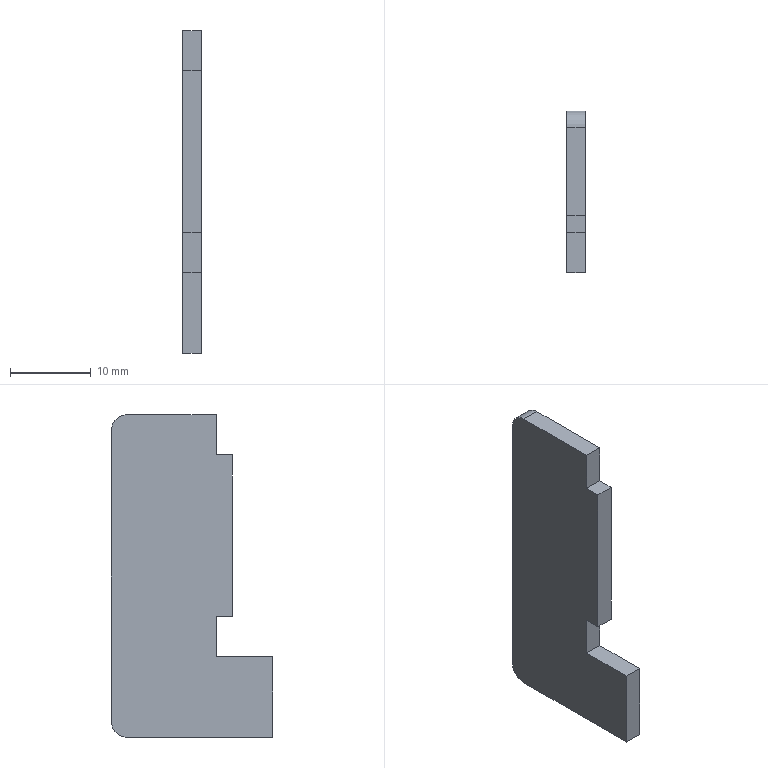Part | SolidWorks | features FlatPattern 1, SMBaseFlange 1, SheetMetal 1 | 1 solid | 14 faces | box 2.3 x 20 x 40 mm | volume 1445 mm3 | plane 12 | cylinder 2 | commonest cylinder face diameters 4 x2
STEP:
#1=CARTESIAN_POINT('',(0.,0.,10.));
#2=VERTEX_POINT('',#1);
#3=CARTESIAN_POINT('',(0.,0.,0.));
#4=VERTEX_POINT('',#3);
#5=CARTESIAN_POINT('',(0.,0.,10.));
#6=DIRECTION('',(0.,0.,-1.));
#7=VECTOR('',#6,1000.);
#8=LINE('',#5,#7);
#9=EDGE_CURVE('',#2,#4,#8,.T.);
#10=ORIENTED_EDGE('',*,*,#9,.F.);
#11=CARTESIAN_POINT('',(-2.3,0.,10.));
#12=VERTEX_POINT('',#11);
#13=CARTESIAN_POINT('',(-2.3,0.,10.));
#14=DIRECTION('',(1.,0.,0.));
#15=VECTOR('',#14,1000.);
#16=LINE('',#13,#15);
#17=EDGE_CURVE('',#12,#2,#16,.T.);
#18=ORIENTED_EDGE('',*,*,#17,.F.);
#19=CARTESIAN_POINT('',(-2.3,0.,0.));
#20=VERTEX_POINT('',#19);
#21=CARTESIAN_POINT('',(-2.3,0.,10.));
#22=DIRECTION('',(0.,0.,-1.));
#23=VECTOR('',#22,1000.);
#24=LINE('',#21,#23);
#25=EDGE_CURVE('',#12,#20,#24,.T.);
#26=ORIENTED_EDGE('',*,*,#25,.T.);
#27=CARTESIAN_POINT('',(-2.3,0.,0.));
#28=DIRECTION('',(1.,0.,0.));
#29=VECTOR('',#28,1000.);
#30=LINE('',#27,#29);
#31=EDGE_CURVE('',#20,#4,#30,.T.);
#32=ORIENTED_EDGE('',*,*,#31,.T.);
#33=EDGE_LOOP('',(#10,#18,#26,#32));
#34=FACE_OUTER_BOUND('',#33,.T.);
#35=CARTESIAN_POINT('',(-2.3,0.,10.));
#36=DIRECTION('',(0.,-1.,0.));
#37=DIRECTION('',(0.,0.,-1.));
#38=AXIS2_PLACEMENT_3D('',#35,#36,#37);
#39=PLANE('',#38);
#40=ADVANCED_FACE('',(#34),#39,.T.);
#41=CARTESIAN_POINT('',(0.,7.,10.));
#42=VERTEX_POINT('',#41);
#43=CARTESIAN_POINT('',(0.,7.,10.));
#44=DIRECTION('',(0.,-1.,0.));
#45=VECTOR('',#44,1000.);
#46=LINE('',#43,#45);
#47=EDGE_CURVE('',#42,#2,#46,.T.);
#48=ORIENTED_EDGE('',*,*,#47,.F.);
#49=CARTESIAN_POINT('',(-2.3,7.,10.));
#50=VERTEX_POINT('',#49);
#51=CARTESIAN_POINT('',(-2.3,7.,10.));
#52=DIRECTION('',(1.,0.,0.));
#53=VECTOR('',#52,1000.);
#54=LINE('',#51,#53);
#55=EDGE_CURVE('',#50,#42,#54,.T.);
#56=ORIENTED_EDGE('',*,*,#55,.F.);
#57=CARTESIAN_POINT('',(-2.3,7.,10.));
#58=DIRECTION('',(0.,-1.,0.));
#59=VECTOR('',#58,1000.);
#60=LINE('',#57,#59);
#61=EDGE_CURVE('',#50,#12,#60,.T.);
#62=ORIENTED_EDGE('',*,*,#61,.T.);
#63=ORIENTED_EDGE('',*,*,#17,.T.);
#64=EDGE_LOOP('',(#48,#56,#62,#63));
#65=FACE_OUTER_BOUND('',#64,.T.);
#66=CARTESIAN_POINT('',(-2.3,7.,10.));
#67=DIRECTION('',(0.,0.,1.));
#68=DIRECTION('',(0.,-1.,0.));
#69=AXIS2_PLACEMENT_3D('',#66,#67,#68);
#70=PLANE('',#69);
#71=ADVANCED_FACE('',(#65),#70,.T.);
#72=CARTESIAN_POINT('',(0.,7.,15.));
#73=VERTEX_POINT('',#72);
#74=CARTESIAN_POINT('',(0.,7.,15.));
#75=DIRECTION('',(0.,0.,-1.));
#76=VECTOR('',#75,1000.);
#77=LINE('',#74,#76);
#78=EDGE_CURVE('',#73,#42,#77,.T.);
#79=ORIENTED_EDGE('',*,*,#78,.F.);
#80=CARTESIAN_POINT('',(-2.3,7.,15.));
#81=VERTEX_POINT('',#80);
#82=CARTESIAN_POINT('',(-2.3,7.,15.));
#83=DIRECTION('',(1.,0.,0.));
#84=VECTOR('',#83,1000.);
#85=LINE('',#82,#84);
#86=EDGE_CURVE('',#81,#73,#85,.T.);
#87=ORIENTED_EDGE('',*,*,#86,.F.);
#88=CARTESIAN_POINT('',(-2.3,7.,15.));
#89=DIRECTION('',(0.,0.,-1.));
#90=VECTOR('',#89,1000.);
#91=LINE('',#88,#90);
#92=EDGE_CURVE('',#81,#50,#91,.T.);
#93=ORIENTED_EDGE('',*,*,#92,.T.);
#94=ORIENTED_EDGE('',*,*,#55,.T.);
#95=EDGE_LOOP('',(#79,#87,#93,#94));
#96=FACE_OUTER_BOUND('',#95,.T.);
#97=CARTESIAN_POINT('',(-2.3,7.,15.));
#98=DIRECTION('',(0.,-1.,0.));
#99=DIRECTION('',(0.,0.,-1.));
#100=AXIS2_PLACEMENT_3D('',#97,#98,#99);
#101=PLANE('',#100);
#102=ADVANCED_FACE('',(#96),#101,.T.);
#103=CARTESIAN_POINT('',(0.,5.,15.));
#104=VERTEX_POINT('',#103);
#105=CARTESIAN_POINT('',(0.,5.,15.));
#106=DIRECTION('',(0.,1.,0.));
#107=VECTOR('',#106,1000.);
#108=LINE('',#105,#107);
#109=EDGE_CURVE('',#104,#73,#108,.T.);
#110=ORIENTED_EDGE('',*,*,#109,.F.);
#111=CARTESIAN_POINT('',(-2.3,5.,15.));
#112=VERTEX_POINT('',#111);
#113=CARTESIAN_POINT('',(-2.3,5.,15.));
#114=DIRECTION('',(1.,0.,0.));
#115=VECTOR('',#114,1000.);
#116=LINE('',#113,#115);
#117=EDGE_CURVE('',#112,#104,#116,.T.);
#118=ORIENTED_EDGE('',*,*,#117,.F.);
#119=CARTESIAN_POINT('',(-2.3,5.,15.));
#120=DIRECTION('',(0.,1.,0.));
#121=VECTOR('',#120,1000.);
#122=LINE('',#119,#121);
#123=EDGE_CURVE('',#112,#81,#122,.T.);
#124=ORIENTED_EDGE('',*,*,#123,.T.);
#125=ORIENTED_EDGE('',*,*,#86,.T.);
#126=EDGE_LOOP('',(#110,#118,#124,#125));
#127=FACE_OUTER_BOUND('',#126,.T.);
#128=CARTESIAN_POINT('',(-2.3,5.,15.));
#129=DIRECTION('',(0.,0.,-1.));
#130=DIRECTION('',(-1.,0.,0.));
#131=AXIS2_PLACEMENT_3D('',#128,#129,#130);
#132=PLANE('',#131);
#133=ADVANCED_FACE('',(#127),#132,.T.);
#134=CARTESIAN_POINT('',(0.,5.,35.));
#135=VERTEX_POINT('',#134);
#136=CARTESIAN_POINT('',(0.,5.,35.));
#137=DIRECTION('',(0.,0.,-1.));
#138=VECTOR('',#137,1000.);
#139=LINE('',#136,#138);
#140=EDGE_CURVE('',#135,#104,#139,.T.);
#141=ORIENTED_EDGE('',*,*,#140,.F.);
#142=CARTESIAN_POINT('',(-2.3,5.,35.));
#143=VERTEX_POINT('',#142);
#144=CARTESIAN_POINT('',(-2.3,5.,35.));
#145=DIRECTION('',(1.,0.,0.));
#146=VECTOR('',#145,1000.);
#147=LINE('',#144,#146);
#148=EDGE_CURVE('',#143,#135,#147,.T.);
#149=ORIENTED_EDGE('',*,*,#148,.F.);
#150=CARTESIAN_POINT('',(-2.3,5.,35.));
#151=DIRECTION('',(0.,0.,-1.));
#152=VECTOR('',#151,1000.);
#153=LINE('',#150,#152);
#154=EDGE_CURVE('',#143,#112,#153,.T.);
#155=ORIENTED_EDGE('',*,*,#154,.T.);
#156=ORIENTED_EDGE('',*,*,#117,.T.);
#157=EDGE_LOOP('',(#141,#149,#155,#156));
#158=FACE_OUTER_BOUND('',#157,.T.);
#159=CARTESIAN_POINT('',(-2.3,5.,35.));
#160=DIRECTION('',(0.,-1.,0.));
#161=DIRECTION('',(0.,0.,-1.));
#162=AXIS2_PLACEMENT_3D('',#159,#160,#161);
#163=PLANE('',#162);
#164=ADVANCED_FACE('',(#158),#163,.T.);
#165=CARTESIAN_POINT('',(0.,7.,35.));
#166=VERTEX_POINT('',#165);
#167=CARTESIAN_POINT('',(0.,7.,35.));
#168=DIRECTION('',(0.,-1.,0.));
#169=VECTOR('',#168,1000.);
#170=LINE('',#167,#169);
#171=EDGE_CURVE('',#166,#135,#170,.T.);
#172=ORIENTED_EDGE('',*,*,#171,.F.);
#173=CARTESIAN_POINT('',(-2.3,7.,35.));
#174=VERTEX_POINT('',#173);
#175=CARTESIAN_POINT('',(-2.3,7.,35.));
#176=DIRECTION('',(1.,0.,0.));
#177=VECTOR('',#176,1000.);
#178=LINE('',#175,#177);
#179=EDGE_CURVE('',#174,#166,#178,.T.);
#180=ORIENTED_EDGE('',*,*,#179,.F.);
#181=CARTESIAN_POINT('',(-2.3,7.,35.));
#182=DIRECTION('',(0.,-1.,0.));
#183=VECTOR('',#182,1000.);
#184=LINE('',#181,#183);
#185=EDGE_CURVE('',#174,#143,#184,.T.);
#186=ORIENTED_EDGE('',*,*,#185,.T.);
#187=ORIENTED_EDGE('',*,*,#148,.T.);
#188=EDGE_LOOP('',(#172,#180,#186,#187));
#189=FACE_OUTER_BOUND('',#188,.T.);
#190=CARTESIAN_POINT('',(-2.3,7.,35.));
#191=DIRECTION('',(0.,0.,1.));
#192=DIRECTION('',(1.,0.,0.));
#193=AXIS2_PLACEMENT_3D('',#190,#191,#192);
#194=PLANE('',#193);
#195=ADVANCED_FACE('',(#189),#194,.T.);
#196=CARTESIAN_POINT('',(0.,7.,40.));
#197=VERTEX_POINT('',#196);
#198=CARTESIAN_POINT('',(0.,7.,40.));
#199=DIRECTION('',(0.,0.,-1.));
#200=VECTOR('',#199,1000.);
#201=LINE('',#198,#200);
#202=EDGE_CURVE('',#197,#166,#201,.T.);
#203=ORIENTED_EDGE('',*,*,#202,.F.);
#204=CARTESIAN_POINT('',(-2.3,7.,40.));
#205=VERTEX_POINT('',#204);
#206=CARTESIAN_POINT('',(-2.3,7.,40.));
#207=DIRECTION('',(1.,0.,0.));
#208=VECTOR('',#207,1000.);
#209=LINE('',#206,#208);
#210=EDGE_CURVE('',#205,#197,#209,.T.);
#211=ORIENTED_EDGE('',*,*,#210,.F.);
#212=CARTESIAN_POINT('',(-2.3,7.,40.));
#213=DIRECTION('',(0.,0.,-1.));
#214=VECTOR('',#213,1000.);
#215=LINE('',#212,#214);
#216=EDGE_CURVE('',#205,#174,#215,.T.);
#217=ORIENTED_EDGE('',*,*,#216,.T.);
#218=ORIENTED_EDGE('',*,*,#179,.T.);
#219=EDGE_LOOP('',(#203,#211,#217,#218));
#220=FACE_OUTER_BOUND('',#219,.T.);
#221=CARTESIAN_POINT('',(-2.3,7.,40.));
#222=DIRECTION('',(0.,-1.,0.));
#223=DIRECTION('',(0.,0.,-1.));
#224=AXIS2_PLACEMENT_3D('',#221,#222,#223);
#225=PLANE('',#224);
#226=ADVANCED_FACE('',(#220),#225,.T.);
#227=CARTESIAN_POINT('',(0.,18.,40.));
#228=VERTEX_POINT('',#227);
#229=CARTESIAN_POINT('',(0.,18.,40.));
#230=DIRECTION('',(0.,-1.,0.));
#231=VECTOR('',#230,1000.);
#232=LINE('',#229,#231);
#233=EDGE_CURVE('',#228,#197,#232,.T.);
#234=ORIENTED_EDGE('',*,*,#233,.F.);
#235=CARTESIAN_POINT('',(-2.3,18.,40.));
#236=VERTEX_POINT('',#235);
#237=CARTESIAN_POINT('',(-2.3,18.,40.));
#238=DIRECTION('',(1.,0.,0.));
#239=VECTOR('',#238,1000.);
#240=LINE('',#237,#239);
#241=EDGE_CURVE('',#236,#228,#240,.T.);
#242=ORIENTED_EDGE('',*,*,#241,.F.);
#243=CARTESIAN_POINT('',(-2.3,18.,40.));
#244=DIRECTION('',(0.,-1.,0.));
#245=VECTOR('',#244,1000.);
#246=LINE('',#243,#245);
#247=EDGE_CURVE('',#236,#205,#246,.T.);
#248=ORIENTED_EDGE('',*,*,#247,.T.);
#249=ORIENTED_EDGE('',*,*,#210,.T.);
#250=EDGE_LOOP('',(#234,#242,#248,#249));
#251=FACE_OUTER_BOUND('',#250,.T.);
#252=CARTESIAN_POINT('',(-2.3,18.,40.));
#253=DIRECTION('',(0.,0.,1.));
#254=DIRECTION('',(1.,0.,0.));
#255=AXIS2_PLACEMENT_3D('',#252,#253,#254);
#256=PLANE('',#255);
#257=ADVANCED_FACE('',(#251),#256,.T.);
#258=CARTESIAN_POINT('',(0.,20.,38.));
#259=VERTEX_POINT('',#258);
#260=CARTESIAN_POINT('',(0.,18.,38.));
#261=DIRECTION('',(1.,0.,0.));
#262=DIRECTION('',(0.,0.,-1.));
#263=AXIS2_PLACEMENT_3D('',#260,#261,#262);
#264=CIRCLE('',#263,2.);
#265=EDGE_CURVE('',#259,#228,#264,.T.);
#266=ORIENTED_EDGE('',*,*,#265,.F.);
#267=CARTESIAN_POINT('',(-2.3,20.,38.));
#268=VERTEX_POINT('',#267);
#269=CARTESIAN_POINT('',(-2.3,20.,38.));
#270=DIRECTION('',(1.,0.,0.));
#271=VECTOR('',#270,1000.);
#272=LINE('',#269,#271);
#273=EDGE_CURVE('',#268,#259,#272,.T.);
#274=ORIENTED_EDGE('',*,*,#273,.F.);
#275=CARTESIAN_POINT('',(-2.3,18.,38.));
#276=DIRECTION('',(1.,0.,0.));
#277=DIRECTION('',(0.,0.,-1.));
#278=AXIS2_PLACEMENT_3D('',#275,#276,#277);
#279=CIRCLE('',#278,2.);
#280=EDGE_CURVE('',#268,#236,#279,.T.);
#281=ORIENTED_EDGE('',*,*,#280,.T.);
#282=ORIENTED_EDGE('',*,*,#241,.T.);
#283=EDGE_LOOP('',(#266,#274,#281,#282));
#284=FACE_OUTER_BOUND('',#283,.T.);
#285=CARTESIAN_POINT('',(-2.3,18.,38.));
#286=DIRECTION('',(1.,0.,0.));
#287=DIRECTION('',(0.,0.,-1.));
#288=AXIS2_PLACEMENT_3D('',#285,#286,#287);
#289=CYLINDRICAL_SURFACE('',#288,2.);
#290=ADVANCED_FACE('',(#284),#289,.T.);
#291=CARTESIAN_POINT('',(0.,20.,2.));
#292=VERTEX_POINT('',#291);
#293=CARTESIAN_POINT('',(0.,20.,2.));
#294=DIRECTION('',(0.,0.,1.));
#295=VECTOR('',#294,1000.);
#296=LINE('',#293,#295);
#297=EDGE_CURVE('',#292,#259,#296,.T.);
#298=ORIENTED_EDGE('',*,*,#297,.F.);
#299=CARTESIAN_POINT('',(-2.3,20.,2.));
#300=VERTEX_POINT('',#299);
#301=CARTESIAN_POINT('',(-2.3,20.,2.));
#302=DIRECTION('',(1.,0.,0.));
#303=VECTOR('',#302,1000.);
#304=LINE('',#301,#303);
#305=EDGE_CURVE('',#300,#292,#304,.T.);
#306=ORIENTED_EDGE('',*,*,#305,.F.);
#307=CARTESIAN_POINT('',(-2.3,20.,2.));
#308=DIRECTION('',(0.,0.,1.));
#309=VECTOR('',#308,1000.);
#310=LINE('',#307,#309);
#311=EDGE_CURVE('',#300,#268,#310,.T.);
#312=ORIENTED_EDGE('',*,*,#311,.T.);
#313=ORIENTED_EDGE('',*,*,#273,.T.);
#314=EDGE_LOOP('',(#298,#306,#312,#313));
#315=FACE_OUTER_BOUND('',#314,.T.);
#316=CARTESIAN_POINT('',(-2.3,20.,2.));
#317=DIRECTION('',(0.,1.,0.));
#318=DIRECTION('',(0.,0.,1.));
#319=AXIS2_PLACEMENT_3D('',#316,#317,#318);
#320=PLANE('',#319);
#321=ADVANCED_FACE('',(#315),#320,.T.);
#322=CARTESIAN_POINT('',(0.,18.,0.));
#323=VERTEX_POINT('',#322);
#324=CARTESIAN_POINT('',(0.,18.,2.));
#325=DIRECTION('',(1.,0.,0.));
#326=DIRECTION('',(0.,0.,-1.));
#327=AXIS2_PLACEMENT_3D('',#324,#325,#326);
#328=CIRCLE('',#327,2.);
#329=EDGE_CURVE('',#323,#292,#328,.T.);
#330=ORIENTED_EDGE('',*,*,#329,.F.);
#331=CARTESIAN_POINT('',(-2.3,18.,0.));
#332=VERTEX_POINT('',#331);
#333=CARTESIAN_POINT('',(-2.3,18.,0.));
#334=DIRECTION('',(1.,0.,0.));
#335=VECTOR('',#334,1000.);
#336=LINE('',#333,#335);
#337=EDGE_CURVE('',#332,#323,#336,.T.);
#338=ORIENTED_EDGE('',*,*,#337,.F.);
#339=CARTESIAN_POINT('',(-2.3,18.,2.));
#340=DIRECTION('',(1.,0.,0.));
#341=DIRECTION('',(0.,0.,-1.));
#342=AXIS2_PLACEMENT_3D('',#339,#340,#341);
#343=CIRCLE('',#342,2.);
#344=EDGE_CURVE('',#332,#300,#343,.T.);
#345=ORIENTED_EDGE('',*,*,#344,.T.);
#346=ORIENTED_EDGE('',*,*,#305,.T.);
#347=EDGE_LOOP('',(#330,#338,#345,#346));
#348=FACE_OUTER_BOUND('',#347,.T.);
#349=CARTESIAN_POINT('',(-2.3,18.,2.));
#350=DIRECTION('',(1.,0.,0.));
#351=DIRECTION('',(0.,0.,-1.));
#352=AXIS2_PLACEMENT_3D('',#349,#350,#351);
#353=CYLINDRICAL_SURFACE('',#352,2.);
#354=ADVANCED_FACE('',(#348),#353,.T.);
#355=CARTESIAN_POINT('',(0.,0.,0.));
#356=DIRECTION('',(0.,1.,0.));
#357=VECTOR('',#356,1000.);
#358=LINE('',#355,#357);
#359=EDGE_CURVE('',#4,#323,#358,.T.);
#360=ORIENTED_EDGE('',*,*,#359,.F.);
#361=ORIENTED_EDGE('',*,*,#31,.F.);
#362=CARTESIAN_POINT('',(-2.3,0.,0.));
#363=DIRECTION('',(0.,1.,0.));
#364=VECTOR('',#363,1000.);
#365=LINE('',#362,#364);
#366=EDGE_CURVE('',#20,#332,#365,.T.);
#367=ORIENTED_EDGE('',*,*,#366,.T.);
#368=ORIENTED_EDGE('',*,*,#337,.T.);
#369=EDGE_LOOP('',(#360,#361,#367,#368));
#370=FACE_OUTER_BOUND('',#369,.T.);
#371=CARTESIAN_POINT('',(-2.3,0.,0.));
#372=DIRECTION('',(0.,0.,-1.));
#373=DIRECTION('',(0.,1.,0.));
#374=AXIS2_PLACEMENT_3D('',#371,#372,#373);
#375=PLANE('',#374);
#376=ADVANCED_FACE('',(#370),#375,.T.);
#377=ORIENTED_EDGE('',*,*,#25,.F.);
#378=ORIENTED_EDGE('',*,*,#61,.F.);
#379=ORIENTED_EDGE('',*,*,#92,.F.);
#380=ORIENTED_EDGE('',*,*,#123,.F.);
#381=ORIENTED_EDGE('',*,*,#154,.F.);
#382=ORIENTED_EDGE('',*,*,#185,.F.);
#383=ORIENTED_EDGE('',*,*,#216,.F.);
#384=ORIENTED_EDGE('',*,*,#247,.F.);
#385=ORIENTED_EDGE('',*,*,#280,.F.);
#386=ORIENTED_EDGE('',*,*,#311,.F.);
#387=ORIENTED_EDGE('',*,*,#344,.F.);
#388=ORIENTED_EDGE('',*,*,#366,.F.);
#389=EDGE_LOOP('',(#377,#378,#379,#380,#381,#382,#383,#384,#385,#386,#387,#388));
#390=FACE_OUTER_BOUND('',#389,.T.);
#391=CARTESIAN_POINT('',(-2.3,18.,2.));
#392=DIRECTION('',(1.,0.,0.));
#393=DIRECTION('',(0.,0.,-1.));
#394=AXIS2_PLACEMENT_3D('',#391,#392,#393);
#395=PLANE('',#394);
#396=ADVANCED_FACE('',(#390),#395,.F.);
#397=ORIENTED_EDGE('',*,*,#9,.T.);
#398=ORIENTED_EDGE('',*,*,#359,.T.);
#399=ORIENTED_EDGE('',*,*,#329,.T.);
#400=ORIENTED_EDGE('',*,*,#297,.T.);
#401=ORIENTED_EDGE('',*,*,#265,.T.);
#402=ORIENTED_EDGE('',*,*,#233,.T.);
#403=ORIENTED_EDGE('',*,*,#202,.T.);
#404=ORIENTED_EDGE('',*,*,#171,.T.);
#405=ORIENTED_EDGE('',*,*,#140,.T.);
#406=ORIENTED_EDGE('',*,*,#109,.T.);
#407=ORIENTED_EDGE('',*,*,#78,.T.);
#408=ORIENTED_EDGE('',*,*,#47,.T.);
#409=EDGE_LOOP('',(#397,#398,#399,#400,#401,#402,#403,#404,#405,#406,#407,#408));
#410=FACE_OUTER_BOUND('',#409,.T.);
#411=CARTESIAN_POINT('',(0.,18.,2.));
#412=DIRECTION('',(1.,0.,0.));
#413=DIRECTION('',(0.,0.,-1.));
#414=AXIS2_PLACEMENT_3D('',#411,#412,#413);
#415=PLANE('',#414);
#416=ADVANCED_FACE('',(#410),#415,.T.);
#417=CLOSED_SHELL('',(#40,#71,#102,#133,#164,#195,#226,#257,#290,#321,#354,#376,#396,#416));
#418=MANIFOLD_SOLID_BREP('',#417);
#419=CARTESIAN_POINT('',(0.,0.,0.));
#420=DIRECTION('',(0.,0.,1.));
#421=DIRECTION('',(1.,0.,0.));
#422=AXIS2_PLACEMENT_3D('',#419,#420,#421);
#423=(LENGTH_UNIT()NAMED_UNIT(*)SI_UNIT(.MILLI.,.METRE.));
#424=UNCERTAINTY_MEASURE_WITH_UNIT(LENGTH_MEASURE(0.00001),#423,'','');
#425=(NAMED_UNIT(*)PLANE_ANGLE_UNIT()SI_UNIT($,.RADIAN.));
#426=(NAMED_UNIT(*)SI_UNIT($,.STERADIAN.)SOLID_ANGLE_UNIT());
#427=(GEOMETRIC_REPRESENTATION_CONTEXT(3)GLOBAL_UNCERTAINTY_ASSIGNED_CONTEXT((#424))GLOBAL_UNIT_ASSIGNED_CONTEXT((#423,#425,#426))REPRESENTATION_CONTEXT('',''));
#428=ADVANCED_BREP_SHAPE_REPRESENTATION('',(#418,#422),#427);